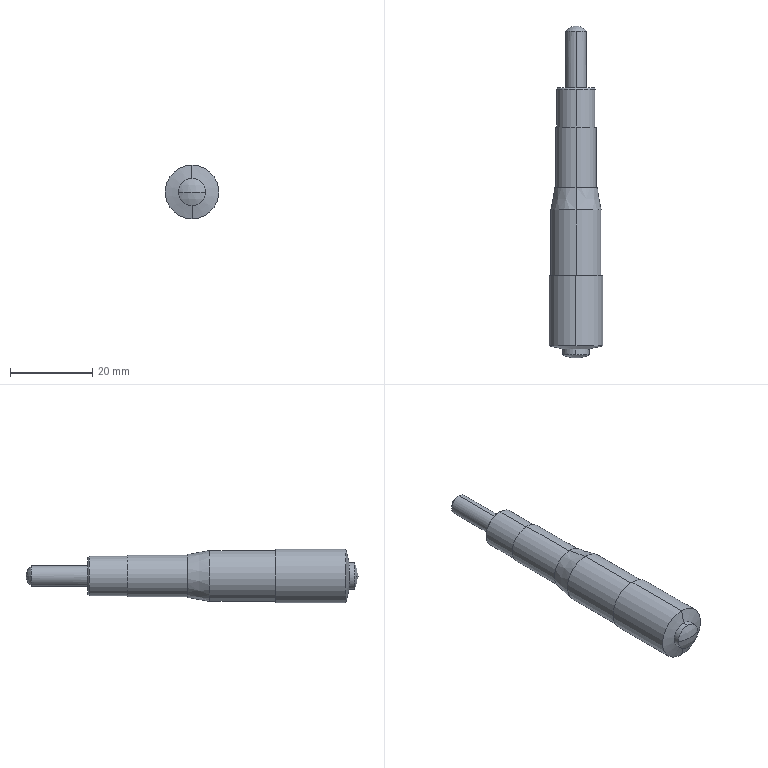Part | STEP file | E-EIC31-80-003 | 1 solid | 26 faces | box 13 x 80.5 x 13 mm | volume 6930 mm3 | cylinder 12 | cone 6 | sphere 4 | plane 4 | commonest cylinder face diameters 5 x2 6.5 x2 9.5 x2 10 x2 12.3 x2 13 x2
STEP:
#1=CARTESIAN_POINT('',(0.,78.429,2.5));
#2=VERTEX_POINT('',#1);
#3=CARTESIAN_POINT('',(2.5,78.429,0.));
#4=VERTEX_POINT('',#3);
#5=CARTESIAN_POINT('',(0.,78.429,0.));
#6=DIRECTION('',(0.,1.,0.));
#7=DIRECTION('',(-1.,0.,0.));
#8=AXIS2_PLACEMENT_3D('',#5,#6,#7);
#9=CIRCLE('',#8,2.5);
#10=EDGE_CURVE('',#2,#4,#9,.T.);
#11=ORIENTED_EDGE('',*,*,#10,.T.);
#12=CARTESIAN_POINT('',(0.,79.724,0.));
#13=VERTEX_POINT('',#12);
#14=CARTESIAN_POINT('',(0.,76.664,0.));
#15=DIRECTION('',(0.,0.,1.));
#16=DIRECTION('',(1.,0.,0.));
#17=AXIS2_PLACEMENT_3D('',#14,#15,#16);
#18=CIRCLE('',#17,3.06);
#19=EDGE_CURVE('',#4,#13,#18,.T.);
#20=ORIENTED_EDGE('',*,*,#19,.T.);
#21=CARTESIAN_POINT('',(-2.5,78.429,0.));
#22=VERTEX_POINT('',#21);
#23=CARTESIAN_POINT('',(0.,76.664,0.));
#24=DIRECTION('',(0.,0.,-1.));
#25=DIRECTION('',(-1.,0.,0.));
#26=AXIS2_PLACEMENT_3D('',#23,#24,#25);
#27=CIRCLE('',#26,3.06);
#28=EDGE_CURVE('',#22,#13,#27,.T.);
#29=ORIENTED_EDGE('',*,*,#28,.F.);
#30=CARTESIAN_POINT('',(0.,78.429,0.));
#31=DIRECTION('',(0.,1.,0.));
#32=DIRECTION('',(-1.,0.,0.));
#33=AXIS2_PLACEMENT_3D('',#30,#31,#32);
#34=CIRCLE('',#33,2.5);
#35=EDGE_CURVE('',#22,#2,#34,.T.);
#36=ORIENTED_EDGE('',*,*,#35,.T.);
#37=EDGE_LOOP('',(#11,#20,#29,#36));
#38=FACE_OUTER_BOUND('',#37,.T.);
#39=CARTESIAN_POINT('',(0.,76.664,0.));
#40=DIRECTION('',(0.,0.,1.));
#41=DIRECTION('',(-1.,0.,0.));
#42=AXIS2_PLACEMENT_3D('',#39,#40,#41);
#43=SPHERICAL_SURFACE('',#42,3.06);
#44=ADVANCED_FACE('',(#38),#43,.T.);
#45=CARTESIAN_POINT('',(0.,64.724,-2.5));
#46=VERTEX_POINT('',#45);
#47=CARTESIAN_POINT('',(0.,64.724,2.5));
#48=VERTEX_POINT('',#47);
#49=CARTESIAN_POINT('',(0.,64.724,0.));
#50=DIRECTION('',(0.,1.,0.));
#51=DIRECTION('',(0.,0.,1.));
#52=AXIS2_PLACEMENT_3D('',#49,#50,#51);
#53=CIRCLE('',#52,2.5);
#54=EDGE_CURVE('',#46,#48,#53,.T.);
#55=ORIENTED_EDGE('',*,*,#54,.T.);
#56=CARTESIAN_POINT('',(0.,50.,2.5));
#57=DIRECTION('',(0.,1.,0.));
#58=VECTOR('',#57,1000.);
#59=LINE('',#56,#58);
#60=EDGE_CURVE('',#48,#2,#59,.T.);
#61=ORIENTED_EDGE('',*,*,#60,.T.);
#62=ORIENTED_EDGE('',*,*,#35,.F.);
#63=CARTESIAN_POINT('',(0.,78.429,-2.5));
#64=VERTEX_POINT('',#63);
#65=CARTESIAN_POINT('',(0.,78.429,0.));
#66=DIRECTION('',(0.,1.,0.));
#67=DIRECTION('',(-1.,0.,0.));
#68=AXIS2_PLACEMENT_3D('',#65,#66,#67);
#69=CIRCLE('',#68,2.5);
#70=EDGE_CURVE('',#64,#22,#69,.T.);
#71=ORIENTED_EDGE('',*,*,#70,.F.);
#72=CARTESIAN_POINT('',(0.,50.,-2.5));
#73=DIRECTION('',(0.,1.,0.));
#74=VECTOR('',#73,1000.);
#75=LINE('',#72,#74);
#76=EDGE_CURVE('',#46,#64,#75,.T.);
#77=ORIENTED_EDGE('',*,*,#76,.F.);
#78=EDGE_LOOP('',(#55,#61,#62,#71,#77));
#79=FACE_OUTER_BOUND('',#78,.T.);
#80=CARTESIAN_POINT('',(0.,50.,0.));
#81=DIRECTION('',(0.,1.,0.));
#82=DIRECTION('',(0.,0.,-1.));
#83=AXIS2_PLACEMENT_3D('',#80,#81,#82);
#84=CYLINDRICAL_SURFACE('',#83,2.5);
#85=ADVANCED_FACE('',(#79),#84,.T.);
#86=CARTESIAN_POINT('',(0.,64.724,-4.45));
#87=VERTEX_POINT('',#86);
#88=CARTESIAN_POINT('',(0.,64.724,4.45));
#89=VERTEX_POINT('',#88);
#90=CARTESIAN_POINT('',(0.,64.724,0.));
#91=DIRECTION('',(0.,1.,0.));
#92=DIRECTION('',(-0.000000143,0.,-1.));
#93=AXIS2_PLACEMENT_3D('',#90,#91,#92);
#94=CIRCLE('',#93,4.45);
#95=EDGE_CURVE('',#87,#89,#94,.T.);
#96=ORIENTED_EDGE('',*,*,#95,.F.);
#97=CARTESIAN_POINT('',(0.,64.424,-4.75));
#98=VERTEX_POINT('',#97);
#99=CARTESIAN_POINT('',(0.,64.424,-4.75));
#100=DIRECTION('',(0.,-0.7071,-0.7071));
#101=VECTOR('',#100,1000.);
#102=LINE('',#99,#101);
#103=EDGE_CURVE('',#87,#98,#102,.T.);
#104=ORIENTED_EDGE('',*,*,#103,.T.);
#105=CARTESIAN_POINT('',(0.,64.424,4.75));
#106=VERTEX_POINT('',#105);
#107=CARTESIAN_POINT('',(0.,64.424,0.));
#108=DIRECTION('',(0.,1.,0.));
#109=DIRECTION('',(0.,0.,1.));
#110=AXIS2_PLACEMENT_3D('',#107,#108,#109);
#111=CIRCLE('',#110,4.75);
#112=EDGE_CURVE('',#98,#106,#111,.T.);
#113=ORIENTED_EDGE('',*,*,#112,.T.);
#114=CARTESIAN_POINT('',(0.,64.424,4.75));
#115=DIRECTION('',(0.,-0.7071,0.7071));
#116=VECTOR('',#115,1000.);
#117=LINE('',#114,#116);
#118=EDGE_CURVE('',#89,#106,#117,.T.);
#119=ORIENTED_EDGE('',*,*,#118,.F.);
#120=EDGE_LOOP('',(#96,#104,#113,#119));
#121=FACE_OUTER_BOUND('',#120,.T.);
#122=CARTESIAN_POINT('',(0.,64.424,0.));
#123=DIRECTION('',(0.,-1.,0.));
#124=DIRECTION('',(0.,0.,1.));
#125=AXIS2_PLACEMENT_3D('',#122,#123,#124);
#126=CONICAL_SURFACE('',#125,4.75,0.7854);
#127=ADVANCED_FACE('',(#121),#126,.T.);
#128=CARTESIAN_POINT('',(0.,55.224,-4.75));
#129=VERTEX_POINT('',#128);
#130=CARTESIAN_POINT('',(0.,55.224,4.75));
#131=VERTEX_POINT('',#130);
#132=CARTESIAN_POINT('',(0.,55.224,0.));
#133=DIRECTION('',(0.,1.,0.));
#134=DIRECTION('',(0.,0.,1.));
#135=AXIS2_PLACEMENT_3D('',#132,#133,#134);
#136=CIRCLE('',#135,4.75);
#137=EDGE_CURVE('',#129,#131,#136,.T.);
#138=ORIENTED_EDGE('',*,*,#137,.T.);
#139=CARTESIAN_POINT('',(0.,50.,4.75));
#140=DIRECTION('',(0.,1.,0.));
#141=VECTOR('',#140,1000.);
#142=LINE('',#139,#141);
#143=EDGE_CURVE('',#131,#106,#142,.T.);
#144=ORIENTED_EDGE('',*,*,#143,.T.);
#145=ORIENTED_EDGE('',*,*,#112,.F.);
#146=CARTESIAN_POINT('',(0.,50.,-4.75));
#147=DIRECTION('',(0.,1.,0.));
#148=VECTOR('',#147,1000.);
#149=LINE('',#146,#148);
#150=EDGE_CURVE('',#129,#98,#149,.T.);
#151=ORIENTED_EDGE('',*,*,#150,.F.);
#152=EDGE_LOOP('',(#138,#144,#145,#151));
#153=FACE_OUTER_BOUND('',#152,.T.);
#154=CARTESIAN_POINT('',(0.,50.,0.));
#155=DIRECTION('',(0.,1.,0.));
#156=DIRECTION('',(0.,0.,-1.));
#157=AXIS2_PLACEMENT_3D('',#154,#155,#156);
#158=CYLINDRICAL_SURFACE('',#157,4.75);
#159=ADVANCED_FACE('',(#153),#158,.T.);
#160=CARTESIAN_POINT('',(0.,40.554,-5.));
#161=VERTEX_POINT('',#160);
#162=CARTESIAN_POINT('',(0.,40.554,5.));
#163=VERTEX_POINT('',#162);
#164=CARTESIAN_POINT('',(0.,40.554,0.));
#165=DIRECTION('',(0.,1.,0.));
#166=DIRECTION('',(0.,0.,1.));
#167=AXIS2_PLACEMENT_3D('',#164,#165,#166);
#168=CIRCLE('',#167,5.);
#169=EDGE_CURVE('',#161,#163,#168,.T.);
#170=ORIENTED_EDGE('',*,*,#169,.T.);
#171=CARTESIAN_POINT('',(0.,55.224,5.));
#172=VERTEX_POINT('',#171);
#173=CARTESIAN_POINT('',(0.,50.,5.));
#174=DIRECTION('',(0.,1.,0.));
#175=VECTOR('',#174,1000.);
#176=LINE('',#173,#175);
#177=EDGE_CURVE('',#163,#172,#176,.T.);
#178=ORIENTED_EDGE('',*,*,#177,.T.);
#179=CARTESIAN_POINT('',(-0.000000709,55.224,-5.));
#180=VERTEX_POINT('',#179);
#181=CARTESIAN_POINT('',(0.,55.224,0.));
#182=DIRECTION('',(0.,1.,0.));
#183=DIRECTION('',(-0.000000142,0.,-1.));
#184=AXIS2_PLACEMENT_3D('',#181,#182,#183);
#185=CIRCLE('',#184,5.);
#186=EDGE_CURVE('',#180,#172,#185,.T.);
#187=ORIENTED_EDGE('',*,*,#186,.F.);
#188=CARTESIAN_POINT('',(0.,50.,-5.));
#189=DIRECTION('',(0.,1.,0.));
#190=VECTOR('',#189,1000.);
#191=LINE('',#188,#190);
#192=EDGE_CURVE('',#161,#180,#191,.T.);
#193=ORIENTED_EDGE('',*,*,#192,.F.);
#194=EDGE_LOOP('',(#170,#178,#187,#193));
#195=FACE_OUTER_BOUND('',#194,.T.);
#196=CARTESIAN_POINT('',(0.,50.,0.));
#197=DIRECTION('',(0.,1.,0.));
#198=DIRECTION('',(0.,0.,-1.));
#199=AXIS2_PLACEMENT_3D('',#196,#197,#198);
#200=CYLINDRICAL_SURFACE('',#199,5.);
#201=ADVANCED_FACE('',(#195),#200,.T.);
#202=CARTESIAN_POINT('',(0.,40.554,-5.2));
#203=VERTEX_POINT('',#202);
#204=CARTESIAN_POINT('',(0.,40.554,5.2));
#205=VERTEX_POINT('',#204);
#206=CARTESIAN_POINT('',(0.,40.554,0.));
#207=DIRECTION('',(0.,1.,0.));
#208=DIRECTION('',(-0.000000141,0.,-1.));
#209=AXIS2_PLACEMENT_3D('',#206,#207,#208);
#210=CIRCLE('',#209,5.2);
#211=EDGE_CURVE('',#203,#205,#210,.T.);
#212=ORIENTED_EDGE('',*,*,#211,.F.);
#213=CARTESIAN_POINT('',(0.,35.154,-6.15));
#214=VERTEX_POINT('',#213);
#215=CARTESIAN_POINT('',(0.,35.154,-6.15));
#216=DIRECTION('',(0.,-0.9849,-0.1733));
#217=VECTOR('',#216,1000.);
#218=LINE('',#215,#217);
#219=EDGE_CURVE('',#203,#214,#218,.T.);
#220=ORIENTED_EDGE('',*,*,#219,.T.);
#221=CARTESIAN_POINT('',(0.,35.154,6.15));
#222=VERTEX_POINT('',#221);
#223=CARTESIAN_POINT('',(0.,35.154,0.));
#224=DIRECTION('',(0.,1.,0.));
#225=DIRECTION('',(0.,0.,1.));
#226=AXIS2_PLACEMENT_3D('',#223,#224,#225);
#227=CIRCLE('',#226,6.15);
#228=EDGE_CURVE('',#214,#222,#227,.T.);
#229=ORIENTED_EDGE('',*,*,#228,.T.);
#230=CARTESIAN_POINT('',(0.,35.154,6.15));
#231=DIRECTION('',(0.,-0.9849,0.1733));
#232=VECTOR('',#231,1000.);
#233=LINE('',#230,#232);
#234=EDGE_CURVE('',#205,#222,#233,.T.);
#235=ORIENTED_EDGE('',*,*,#234,.F.);
#236=EDGE_LOOP('',(#212,#220,#229,#235));
#237=FACE_OUTER_BOUND('',#236,.T.);
#238=CARTESIAN_POINT('',(0.,35.154,0.));
#239=DIRECTION('',(0.,-1.,0.));
#240=DIRECTION('',(0.,0.,1.));
#241=AXIS2_PLACEMENT_3D('',#238,#239,#240);
#242=CONICAL_SURFACE('',#241,6.15,0.1741);
#243=ADVANCED_FACE('',(#237),#242,.T.);
#244=CARTESIAN_POINT('',(0.,19.154,-6.15));
#245=VERTEX_POINT('',#244);
#246=CARTESIAN_POINT('',(0.,19.154,6.15));
#247=VERTEX_POINT('',#246);
#248=CARTESIAN_POINT('',(0.,19.154,0.));
#249=DIRECTION('',(0.,1.,0.));
#250=DIRECTION('',(0.,0.,1.));
#251=AXIS2_PLACEMENT_3D('',#248,#249,#250);
#252=CIRCLE('',#251,6.15);
#253=EDGE_CURVE('',#245,#247,#252,.T.);
#254=ORIENTED_EDGE('',*,*,#253,.T.);
#255=CARTESIAN_POINT('',(0.,50.,6.15));
#256=DIRECTION('',(0.,1.,0.));
#257=VECTOR('',#256,1000.);
#258=LINE('',#255,#257);
#259=EDGE_CURVE('',#247,#222,#258,.T.);
#260=ORIENTED_EDGE('',*,*,#259,.T.);
#261=ORIENTED_EDGE('',*,*,#228,.F.);
#262=CARTESIAN_POINT('',(0.,50.,-6.15));
#263=DIRECTION('',(0.,1.,0.));
#264=VECTOR('',#263,1000.);
#265=LINE('',#262,#264);
#266=EDGE_CURVE('',#245,#214,#265,.T.);
#267=ORIENTED_EDGE('',*,*,#266,.F.);
#268=EDGE_LOOP('',(#254,#260,#261,#267));
#269=FACE_OUTER_BOUND('',#268,.T.);
#270=CARTESIAN_POINT('',(0.,50.,0.));
#271=DIRECTION('',(0.,1.,0.));
#272=DIRECTION('',(0.,0.,-1.));
#273=AXIS2_PLACEMENT_3D('',#270,#271,#272);
#274=CYLINDRICAL_SURFACE('',#273,6.15);
#275=ADVANCED_FACE('',(#269),#274,.T.);
#276=CARTESIAN_POINT('',(0.000000005,2.154,-6.5));
#277=VERTEX_POINT('',#276);
#278=CARTESIAN_POINT('',(-0.000000005,2.154,6.5));
#279=VERTEX_POINT('',#278);
#280=CARTESIAN_POINT('',(0.,2.154,0.));
#281=DIRECTION('',(0.,1.,0.));
#282=DIRECTION('',(0.,0.,1.));
#283=AXIS2_PLACEMENT_3D('',#280,#281,#282);
#284=CIRCLE('',#283,6.5);
#285=EDGE_CURVE('',#277,#279,#284,.T.);
#286=ORIENTED_EDGE('',*,*,#285,.T.);
#287=CARTESIAN_POINT('',(-0.000000005,19.154,6.5));
#288=VERTEX_POINT('',#287);
#289=CARTESIAN_POINT('',(-0.000000005,50.,6.5));
#290=DIRECTION('',(0.,1.,0.));
#291=VECTOR('',#290,1000.);
#292=LINE('',#289,#291);
#293=EDGE_CURVE('',#279,#288,#292,.T.);
#294=ORIENTED_EDGE('',*,*,#293,.T.);
#295=CARTESIAN_POINT('',(0.,19.154,-6.5));
#296=VERTEX_POINT('',#295);
#297=CARTESIAN_POINT('',(0.,19.154,0.));
#298=DIRECTION('',(0.,1.,0.));
#299=DIRECTION('',(0.,0.,-1.));
#300=AXIS2_PLACEMENT_3D('',#297,#298,#299);
#301=CIRCLE('',#300,6.5);
#302=EDGE_CURVE('',#296,#288,#301,.T.);
#303=ORIENTED_EDGE('',*,*,#302,.F.);
#304=CARTESIAN_POINT('',(0.000000005,50.,-6.5));
#305=DIRECTION('',(0.,1.,0.));
#306=VECTOR('',#305,1000.);
#307=LINE('',#304,#306);
#308=EDGE_CURVE('',#277,#296,#307,.T.);
#309=ORIENTED_EDGE('',*,*,#308,.F.);
#310=EDGE_LOOP('',(#286,#294,#303,#309));
#311=FACE_OUTER_BOUND('',#310,.T.);
#312=CARTESIAN_POINT('',(0.,50.,0.));
#313=DIRECTION('',(0.,1.,0.));
#314=DIRECTION('',(0.000000001,0.,-1.));
#315=AXIS2_PLACEMENT_3D('',#312,#313,#314);
#316=CYLINDRICAL_SURFACE('',#315,6.5);
#317=ADVANCED_FACE('',(#311),#316,.T.);
#318=CARTESIAN_POINT('',(0.000000001,1.404,-3.25));
#319=VERTEX_POINT('',#318);
#320=CARTESIAN_POINT('',(-0.000000001,1.404,3.25));
#321=VERTEX_POINT('',#320);
#322=CARTESIAN_POINT('',(0.,1.404,0.));
#323=DIRECTION('',(0.,1.,0.));
#324=DIRECTION('',(0.,0.,1.));
#325=AXIS2_PLACEMENT_3D('',#322,#323,#324);
#326=CIRCLE('',#325,3.25);
#327=EDGE_CURVE('',#319,#321,#326,.T.);
#328=ORIENTED_EDGE('',*,*,#327,.T.);
#329=CARTESIAN_POINT('',(-0.000000005,2.154,6.5));
#330=DIRECTION('',(-0.000000001,0.2249,0.9744));
#331=VECTOR('',#330,1000.);
#332=LINE('',#329,#331);
#333=EDGE_CURVE('',#321,#279,#332,.T.);
#334=ORIENTED_EDGE('',*,*,#333,.T.);
#335=ORIENTED_EDGE('',*,*,#285,.F.);
#336=CARTESIAN_POINT('',(0.000000005,2.154,-6.5));
#337=DIRECTION('',(0.000000001,0.2249,-0.9744));
#338=VECTOR('',#337,1000.);
#339=LINE('',#336,#338);
#340=EDGE_CURVE('',#319,#277,#339,.T.);
#341=ORIENTED_EDGE('',*,*,#340,.F.);
#342=EDGE_LOOP('',(#328,#334,#335,#341));
#343=FACE_OUTER_BOUND('',#342,.T.);
#344=CARTESIAN_POINT('',(0.,2.154,0.));
#345=DIRECTION('',(0.,1.,0.));
#346=DIRECTION('',(0.000000001,0.,-1.));
#347=AXIS2_PLACEMENT_3D('',#344,#345,#346);
#348=CONICAL_SURFACE('',#347,6.5,1.344);
#349=ADVANCED_FACE('',(#343),#348,.T.);
#350=CARTESIAN_POINT('',(-3.25,0.,0.));
#351=VERTEX_POINT('',#350);
#352=CARTESIAN_POINT('',(-0.000000001,0.,3.25));
#353=VERTEX_POINT('',#352);
#354=CARTESIAN_POINT('',(0.,0.,0.));
#355=DIRECTION('',(0.,1.,0.));
#356=DIRECTION('',(-1.,0.,0.));
#357=AXIS2_PLACEMENT_3D('',#354,#355,#356);
#358=CIRCLE('',#357,3.25);
#359=EDGE_CURVE('',#351,#353,#358,.T.);
#360=ORIENTED_EDGE('',*,*,#359,.T.);
#361=CARTESIAN_POINT('',(-0.000000001,50.,3.25));
#362=DIRECTION('',(0.,1.,0.));
#363=VECTOR('',#362,1000.);
#364=LINE('',#361,#363);
#365=EDGE_CURVE('',#353,#321,#364,.T.);
#366=ORIENTED_EDGE('',*,*,#365,.T.);
#367=ORIENTED_EDGE('',*,*,#327,.F.);
#368=CARTESIAN_POINT('',(0.000000001,0.,-3.25));
#369=VERTEX_POINT('',#368);
#370=CARTESIAN_POINT('',(0.000000001,50.,-3.25));
#371=DIRECTION('',(0.,1.,0.));
#372=VECTOR('',#371,1000.);
#373=LINE('',#370,#372);
#374=EDGE_CURVE('',#369,#319,#373,.T.);
#375=ORIENTED_EDGE('',*,*,#374,.F.);
#376=CARTESIAN_POINT('',(0.,0.,0.));
#377=DIRECTION('',(0.,1.,0.));
#378=DIRECTION('',(-1.,0.,0.));
#379=AXIS2_PLACEMENT_3D('',#376,#377,#378);
#380=CIRCLE('',#379,3.25);
#381=EDGE_CURVE('',#369,#351,#380,.T.);
#382=ORIENTED_EDGE('',*,*,#381,.T.);
#383=EDGE_LOOP('',(#360,#366,#367,#375,#382));
#384=FACE_OUTER_BOUND('',#383,.T.);
#385=CARTESIAN_POINT('',(0.,50.,0.));
#386=DIRECTION('',(0.,1.,0.));
#387=DIRECTION('',(0.,0.,-1.));
#388=AXIS2_PLACEMENT_3D('',#385,#386,#387);
#389=CYLINDRICAL_SURFACE('',#388,3.25);
#390=ADVANCED_FACE('',(#384),#389,.T.);
#391=CARTESIAN_POINT('',(0.,-0.7752,0.));
#392=VERTEX_POINT('',#391);
#393=CARTESIAN_POINT('',(3.25,0.,0.));
#394=VERTEX_POINT('',#393);
#395=CARTESIAN_POINT('',(0.,6.425,0.));
#396=DIRECTION('',(0.,0.,1.));
#397=DIRECTION('',(1.,0.,0.));
#398=AXIS2_PLACEMENT_3D('',#395,#396,#397);
#399=CIRCLE('',#398,7.2);
#400=EDGE_CURVE('',#392,#394,#399,.T.);
#401=ORIENTED_EDGE('',*,*,#400,.F.);
#402=CARTESIAN_POINT('',(0.,6.425,0.));
#403=DIRECTION('',(0.,0.,-1.));
#404=DIRECTION('',(-1.,0.,0.));
#405=AXIS2_PLACEMENT_3D('',#402,#403,#404);
#406=CIRCLE('',#405,7.2);
#407=EDGE_CURVE('',#392,#351,#406,.T.);
#408=ORIENTED_EDGE('',*,*,#407,.T.);
#409=ORIENTED_EDGE('',*,*,#381,.F.);
#410=CARTESIAN_POINT('',(0.,0.,0.));
#411=DIRECTION('',(0.,1.,0.));
#412=DIRECTION('',(-1.,0.,0.));
#413=AXIS2_PLACEMENT_3D('',#410,#411,#412);
#414=CIRCLE('',#413,3.25);
#415=EDGE_CURVE('',#394,#369,#414,.T.);
#416=ORIENTED_EDGE('',*,*,#415,.F.);
#417=EDGE_LOOP('',(#401,#408,#409,#416));
#418=FACE_OUTER_BOUND('',#417,.T.);
#419=CARTESIAN_POINT('',(0.,6.425,0.));
#420=DIRECTION('',(0.,0.,-1.));
#421=DIRECTION('',(1.,0.,0.));
#422=AXIS2_PLACEMENT_3D('',#419,#420,#421);
#423=SPHERICAL_SURFACE('',#422,7.2);
#424=ADVANCED_FACE('',(#418),#423,.T.);
#425=ORIENTED_EDGE('',*,*,#302,.T.);
#426=CARTESIAN_POINT('',(0.,19.154,0.));
#427=DIRECTION('',(0.,1.,0.));
#428=DIRECTION('',(0.,0.,-1.));
#429=AXIS2_PLACEMENT_3D('',#426,#427,#428);
#430=CIRCLE('',#429,6.5);
#431=EDGE_CURVE('',#288,#296,#430,.T.);
#432=ORIENTED_EDGE('',*,*,#431,.T.);
#433=EDGE_LOOP('',(#425,#432));
#434=FACE_OUTER_BOUND('',#433,.T.);
#435=ORIENTED_EDGE('',*,*,#253,.F.);
#436=CARTESIAN_POINT('',(0.,19.154,0.));
#437=DIRECTION('',(0.,1.,0.));
#438=DIRECTION('',(0.,0.,1.));
#439=AXIS2_PLACEMENT_3D('',#436,#437,#438);
#440=CIRCLE('',#439,6.15);
#441=EDGE_CURVE('',#247,#245,#440,.T.);
#442=ORIENTED_EDGE('',*,*,#441,.F.);
#443=EDGE_LOOP('',(#435,#442));
#444=FACE_BOUND('',#443,.T.);
#445=CARTESIAN_POINT('',(-6.678,19.154,6.5));
#446=DIRECTION('',(0.,1.,0.));
#447=DIRECTION('',(1.,0.,0.));
#448=AXIS2_PLACEMENT_3D('',#445,#446,#447);
#449=PLANE('',#448);
#450=ADVANCED_FACE('',(#434,#444),#449,.T.);
#451=CARTESIAN_POINT('',(0.,40.554,0.));
#452=DIRECTION('',(0.,1.,0.));
#453=DIRECTION('',(-0.000000141,0.,-1.));
#454=AXIS2_PLACEMENT_3D('',#451,#452,#453);
#455=CIRCLE('',#454,5.2);
#456=EDGE_CURVE('',#205,#203,#455,.T.);
#457=ORIENTED_EDGE('',*,*,#456,.T.);
#458=ORIENTED_EDGE('',*,*,#211,.T.);
#459=EDGE_LOOP('',(#457,#458));
#460=FACE_OUTER_BOUND('',#459,.T.);
#461=ORIENTED_EDGE('',*,*,#169,.F.);
#462=CARTESIAN_POINT('',(0.,40.554,0.));
#463=DIRECTION('',(0.,1.,0.));
#464=DIRECTION('',(0.,0.,1.));
#465=AXIS2_PLACEMENT_3D('',#462,#463,#464);
#466=CIRCLE('',#465,5.);
#467=EDGE_CURVE('',#163,#161,#466,.T.);
#468=ORIENTED_EDGE('',*,*,#467,.F.);
#469=EDGE_LOOP('',(#461,#468));
#470=FACE_BOUND('',#469,.T.);
#471=CARTESIAN_POINT('',(-5.27,40.554,5.2));
#472=DIRECTION('',(0.,1.,0.));
#473=DIRECTION('',(1.,0.,0.));
#474=AXIS2_PLACEMENT_3D('',#471,#472,#473);
#475=PLANE('',#474);
#476=ADVANCED_FACE('',(#460,#470),#475,.T.);
#477=ORIENTED_EDGE('',*,*,#186,.T.);
#478=CARTESIAN_POINT('',(0.,55.224,0.));
#479=DIRECTION('',(0.,1.,0.));
#480=DIRECTION('',(-0.000000142,0.,-1.));
#481=AXIS2_PLACEMENT_3D('',#478,#479,#480);
#482=CIRCLE('',#481,5.);
#483=EDGE_CURVE('',#172,#180,#482,.T.);
#484=ORIENTED_EDGE('',*,*,#483,.T.);
#485=EDGE_LOOP('',(#477,#484));
#486=FACE_OUTER_BOUND('',#485,.T.);
#487=ORIENTED_EDGE('',*,*,#137,.F.);
#488=CARTESIAN_POINT('',(0.,55.224,0.));
#489=DIRECTION('',(0.,1.,0.));
#490=DIRECTION('',(0.,0.,1.));
#491=AXIS2_PLACEMENT_3D('',#488,#489,#490);
#492=CIRCLE('',#491,4.75);
#493=EDGE_CURVE('',#131,#129,#492,.T.);
#494=ORIENTED_EDGE('',*,*,#493,.F.);
#495=EDGE_LOOP('',(#487,#494));
#496=FACE_BOUND('',#495,.T.);
#497=CARTESIAN_POINT('',(-5.,55.224,5.));
#498=DIRECTION('',(0.,1.,0.));
#499=DIRECTION('',(1.,0.,0.));
#500=AXIS2_PLACEMENT_3D('',#497,#498,#499);
#501=PLANE('',#500);
#502=ADVANCED_FACE('',(#486,#496),#501,.T.);
#503=CARTESIAN_POINT('',(0.,64.724,0.));
#504=DIRECTION('',(0.,1.,0.));
#505=DIRECTION('',(-0.000000143,0.,-1.));
#506=AXIS2_PLACEMENT_3D('',#503,#504,#505);
#507=CIRCLE('',#506,4.45);
#508=EDGE_CURVE('',#89,#87,#507,.T.);
#509=ORIENTED_EDGE('',*,*,#508,.T.);
#510=ORIENTED_EDGE('',*,*,#95,.T.);
#511=EDGE_LOOP('',(#509,#510));
#512=FACE_OUTER_BOUND('',#511,.T.);
#513=ORIENTED_EDGE('',*,*,#54,.F.);
#514=CARTESIAN_POINT('',(0.,64.724,0.));
#515=DIRECTION('',(0.,1.,0.));
#516=DIRECTION('',(0.,0.,1.));
#517=AXIS2_PLACEMENT_3D('',#514,#515,#516);
#518=CIRCLE('',#517,2.5);
#519=EDGE_CURVE('',#48,#46,#518,.T.);
#520=ORIENTED_EDGE('',*,*,#519,.F.);
#521=EDGE_LOOP('',(#513,#520));
#522=FACE_BOUND('',#521,.T.);
#523=CARTESIAN_POINT('',(-4.45,64.724,4.45));
#524=DIRECTION('',(0.,1.,0.));
#525=DIRECTION('',(1.,0.,0.));
#526=AXIS2_PLACEMENT_3D('',#523,#524,#525);
#527=PLANE('',#526);
#528=ADVANCED_FACE('',(#512,#522),#527,.T.);
#529=ORIENTED_EDGE('',*,*,#407,.F.);
#530=ORIENTED_EDGE('',*,*,#400,.T.);
#531=CARTESIAN_POINT('',(0.,0.,0.));
#532=DIRECTION('',(0.,1.,0.));
#533=DIRECTION('',(-1.,0.,0.));
#534=AXIS2_PLACEMENT_3D('',#531,#532,#533);
#535=CIRCLE('',#534,3.25);
#536=EDGE_CURVE('',#353,#394,#535,.T.);
#537=ORIENTED_EDGE('',*,*,#536,.F.);
#538=ORIENTED_EDGE('',*,*,#359,.F.);
#539=EDGE_LOOP('',(#529,#530,#537,#538));
#540=FACE_OUTER_BOUND('',#539,.T.);
#541=CARTESIAN_POINT('',(0.,6.425,0.));
#542=DIRECTION('',(0.,0.,-1.));
#543=DIRECTION('',(1.,0.,0.));
#544=AXIS2_PLACEMENT_3D('',#541,#542,#543);
#545=SPHERICAL_SURFACE('',#544,7.2);
#546=ADVANCED_FACE('',(#540),#545,.T.);
#547=ORIENTED_EDGE('',*,*,#365,.F.);
#548=ORIENTED_EDGE('',*,*,#536,.T.);
#549=ORIENTED_EDGE('',*,*,#415,.T.);
#550=ORIENTED_EDGE('',*,*,#374,.T.);
#551=CARTESIAN_POINT('',(0.,1.404,0.));
#552=DIRECTION('',(0.,1.,0.));
#553=DIRECTION('',(0.,0.,1.));
#554=AXIS2_PLACEMENT_3D('',#551,#552,#553);
#555=CIRCLE('',#554,3.25);
#556=EDGE_CURVE('',#321,#319,#555,.T.);
#557=ORIENTED_EDGE('',*,*,#556,.F.);
#558=EDGE_LOOP('',(#547,#548,#549,#550,#557));
#559=FACE_OUTER_BOUND('',#558,.T.);
#560=CARTESIAN_POINT('',(0.,50.,0.));
#561=DIRECTION('',(0.,1.,0.));
#562=DIRECTION('',(0.,0.,-1.));
#563=AXIS2_PLACEMENT_3D('',#560,#561,#562);
#564=CYLINDRICAL_SURFACE('',#563,3.25);
#565=ADVANCED_FACE('',(#559),#564,.T.);
#566=ORIENTED_EDGE('',*,*,#333,.F.);
#567=ORIENTED_EDGE('',*,*,#556,.T.);
#568=ORIENTED_EDGE('',*,*,#340,.T.);
#569=CARTESIAN_POINT('',(0.,2.154,0.));
#570=DIRECTION('',(0.,1.,0.));
#571=DIRECTION('',(0.,0.,1.));
#572=AXIS2_PLACEMENT_3D('',#569,#570,#571);
#573=CIRCLE('',#572,6.5);
#574=EDGE_CURVE('',#279,#277,#573,.T.);
#575=ORIENTED_EDGE('',*,*,#574,.F.);
#576=EDGE_LOOP('',(#566,#567,#568,#575));
#577=FACE_OUTER_BOUND('',#576,.T.);
#578=CARTESIAN_POINT('',(0.,2.154,0.));
#579=DIRECTION('',(0.,1.,0.));
#580=DIRECTION('',(0.000000001,0.,-1.));
#581=AXIS2_PLACEMENT_3D('',#578,#579,#580);
#582=CONICAL_SURFACE('',#581,6.5,1.344);
#583=ADVANCED_FACE('',(#577),#582,.T.);
#584=ORIENTED_EDGE('',*,*,#293,.F.);
#585=ORIENTED_EDGE('',*,*,#574,.T.);
#586=ORIENTED_EDGE('',*,*,#308,.T.);
#587=ORIENTED_EDGE('',*,*,#431,.F.);
#588=EDGE_LOOP('',(#584,#585,#586,#587));
#589=FACE_OUTER_BOUND('',#588,.T.);
#590=CARTESIAN_POINT('',(0.,50.,0.));
#591=DIRECTION('',(0.,1.,0.));
#592=DIRECTION('',(0.000000001,0.,-1.));
#593=AXIS2_PLACEMENT_3D('',#590,#591,#592);
#594=CYLINDRICAL_SURFACE('',#593,6.5);
#595=ADVANCED_FACE('',(#589),#594,.T.);
#596=ORIENTED_EDGE('',*,*,#259,.F.);
#597=ORIENTED_EDGE('',*,*,#441,.T.);
#598=ORIENTED_EDGE('',*,*,#266,.T.);
#599=CARTESIAN_POINT('',(0.,35.154,0.));
#600=DIRECTION('',(0.,1.,0.));
#601=DIRECTION('',(0.,0.,1.));
#602=AXIS2_PLACEMENT_3D('',#599,#600,#601);
#603=CIRCLE('',#602,6.15);
#604=EDGE_CURVE('',#222,#214,#603,.T.);
#605=ORIENTED_EDGE('',*,*,#604,.F.);
#606=EDGE_LOOP('',(#596,#597,#598,#605));
#607=FACE_OUTER_BOUND('',#606,.T.);
#608=CARTESIAN_POINT('',(0.,50.,0.));
#609=DIRECTION('',(0.,1.,0.));
#610=DIRECTION('',(0.,0.,-1.));
#611=AXIS2_PLACEMENT_3D('',#608,#609,#610);
#612=CYLINDRICAL_SURFACE('',#611,6.15);
#613=ADVANCED_FACE('',(#607),#612,.T.);
#614=ORIENTED_EDGE('',*,*,#219,.F.);
#615=ORIENTED_EDGE('',*,*,#456,.F.);
#616=ORIENTED_EDGE('',*,*,#234,.T.);
#617=ORIENTED_EDGE('',*,*,#604,.T.);
#618=EDGE_LOOP('',(#614,#615,#616,#617));
#619=FACE_OUTER_BOUND('',#618,.T.);
#620=CARTESIAN_POINT('',(0.,35.154,0.));
#621=DIRECTION('',(0.,-1.,0.));
#622=DIRECTION('',(0.,0.,1.));
#623=AXIS2_PLACEMENT_3D('',#620,#621,#622);
#624=CONICAL_SURFACE('',#623,6.15,0.1741);
#625=ADVANCED_FACE('',(#619),#624,.T.);
#626=ORIENTED_EDGE('',*,*,#177,.F.);
#627=ORIENTED_EDGE('',*,*,#467,.T.);
#628=ORIENTED_EDGE('',*,*,#192,.T.);
#629=ORIENTED_EDGE('',*,*,#483,.F.);
#630=EDGE_LOOP('',(#626,#627,#628,#629));
#631=FACE_OUTER_BOUND('',#630,.T.);
#632=CARTESIAN_POINT('',(0.,50.,0.));
#633=DIRECTION('',(0.,1.,0.));
#634=DIRECTION('',(0.,0.,-1.));
#635=AXIS2_PLACEMENT_3D('',#632,#633,#634);
#636=CYLINDRICAL_SURFACE('',#635,5.);
#637=ADVANCED_FACE('',(#631),#636,.T.);
#638=ORIENTED_EDGE('',*,*,#143,.F.);
#639=ORIENTED_EDGE('',*,*,#493,.T.);
#640=ORIENTED_EDGE('',*,*,#150,.T.);
#641=CARTESIAN_POINT('',(0.,64.424,0.));
#642=DIRECTION('',(0.,1.,0.));
#643=DIRECTION('',(0.,0.,1.));
#644=AXIS2_PLACEMENT_3D('',#641,#642,#643);
#645=CIRCLE('',#644,4.75);
#646=EDGE_CURVE('',#106,#98,#645,.T.);
#647=ORIENTED_EDGE('',*,*,#646,.F.);
#648=EDGE_LOOP('',(#638,#639,#640,#647));
#649=FACE_OUTER_BOUND('',#648,.T.);
#650=CARTESIAN_POINT('',(0.,50.,0.));
#651=DIRECTION('',(0.,1.,0.));
#652=DIRECTION('',(0.,0.,-1.));
#653=AXIS2_PLACEMENT_3D('',#650,#651,#652);
#654=CYLINDRICAL_SURFACE('',#653,4.75);
#655=ADVANCED_FACE('',(#649),#654,.T.);
#656=ORIENTED_EDGE('',*,*,#103,.F.);
#657=ORIENTED_EDGE('',*,*,#508,.F.);
#658=ORIENTED_EDGE('',*,*,#118,.T.);
#659=ORIENTED_EDGE('',*,*,#646,.T.);
#660=EDGE_LOOP('',(#656,#657,#658,#659));
#661=FACE_OUTER_BOUND('',#660,.T.);
#662=CARTESIAN_POINT('',(0.,64.424,0.));
#663=DIRECTION('',(0.,-1.,0.));
#664=DIRECTION('',(0.,0.,1.));
#665=AXIS2_PLACEMENT_3D('',#662,#663,#664);
#666=CONICAL_SURFACE('',#665,4.75,0.7854);
#667=ADVANCED_FACE('',(#661),#666,.T.);
#668=ORIENTED_EDGE('',*,*,#60,.F.);
#669=ORIENTED_EDGE('',*,*,#519,.T.);
#670=ORIENTED_EDGE('',*,*,#76,.T.);
#671=CARTESIAN_POINT('',(0.,78.429,0.));
#672=DIRECTION('',(0.,1.,0.));
#673=DIRECTION('',(-1.,0.,0.));
#674=AXIS2_PLACEMENT_3D('',#671,#672,#673);
#675=CIRCLE('',#674,2.5);
#676=EDGE_CURVE('',#4,#64,#675,.T.);
#677=ORIENTED_EDGE('',*,*,#676,.F.);
#678=ORIENTED_EDGE('',*,*,#10,.F.);
#679=EDGE_LOOP('',(#668,#669,#670,#677,#678));
#680=FACE_OUTER_BOUND('',#679,.T.);
#681=CARTESIAN_POINT('',(0.,50.,0.));
#682=DIRECTION('',(0.,1.,0.));
#683=DIRECTION('',(0.,0.,-1.));
#684=AXIS2_PLACEMENT_3D('',#681,#682,#683);
#685=CYLINDRICAL_SURFACE('',#684,2.5);
#686=ADVANCED_FACE('',(#680),#685,.T.);
#687=ORIENTED_EDGE('',*,*,#19,.F.);
#688=ORIENTED_EDGE('',*,*,#676,.T.);
#689=ORIENTED_EDGE('',*,*,#70,.T.);
#690=ORIENTED_EDGE('',*,*,#28,.T.);
#691=EDGE_LOOP('',(#687,#688,#689,#690));
#692=FACE_OUTER_BOUND('',#691,.T.);
#693=CARTESIAN_POINT('',(0.,76.664,0.));
#694=DIRECTION('',(0.,0.,1.));
#695=DIRECTION('',(-1.,0.,0.));
#696=AXIS2_PLACEMENT_3D('',#693,#694,#695);
#697=SPHERICAL_SURFACE('',#696,3.06);
#698=ADVANCED_FACE('',(#692),#697,.T.);
#699=CLOSED_SHELL('',(#44,#85,#127,#159,#201,#243,#275,#317,#349,#390,#424,#450,#476,#502,#528,#546,#565,#583,#595,#613,#625,#637,#655,#667,#686,#698));
#700=MANIFOLD_SOLID_BREP('',#699);
#701=CARTESIAN_POINT('',(0.,0.,0.));
#702=DIRECTION('',(0.,0.,1.));
#703=DIRECTION('',(1.,0.,0.));
#704=AXIS2_PLACEMENT_3D('',#701,#702,#703);
#705=(LENGTH_UNIT()NAMED_UNIT(*)SI_UNIT(.MILLI.,.METRE.));
#706=UNCERTAINTY_MEASURE_WITH_UNIT(LENGTH_MEASURE(0.00001),#705,'','');
#707=(NAMED_UNIT(*)PLANE_ANGLE_UNIT()SI_UNIT($,.RADIAN.));
#708=(NAMED_UNIT(*)SI_UNIT($,.STERADIAN.)SOLID_ANGLE_UNIT());
#709=(GEOMETRIC_REPRESENTATION_CONTEXT(3)GLOBAL_UNCERTAINTY_ASSIGNED_CONTEXT((#706))GLOBAL_UNIT_ASSIGNED_CONTEXT((#705,#707,#708))REPRESENTATION_CONTEXT('',''));
#710=ADVANCED_BREP_SHAPE_REPRESENTATION('',(#700,#704),#709);